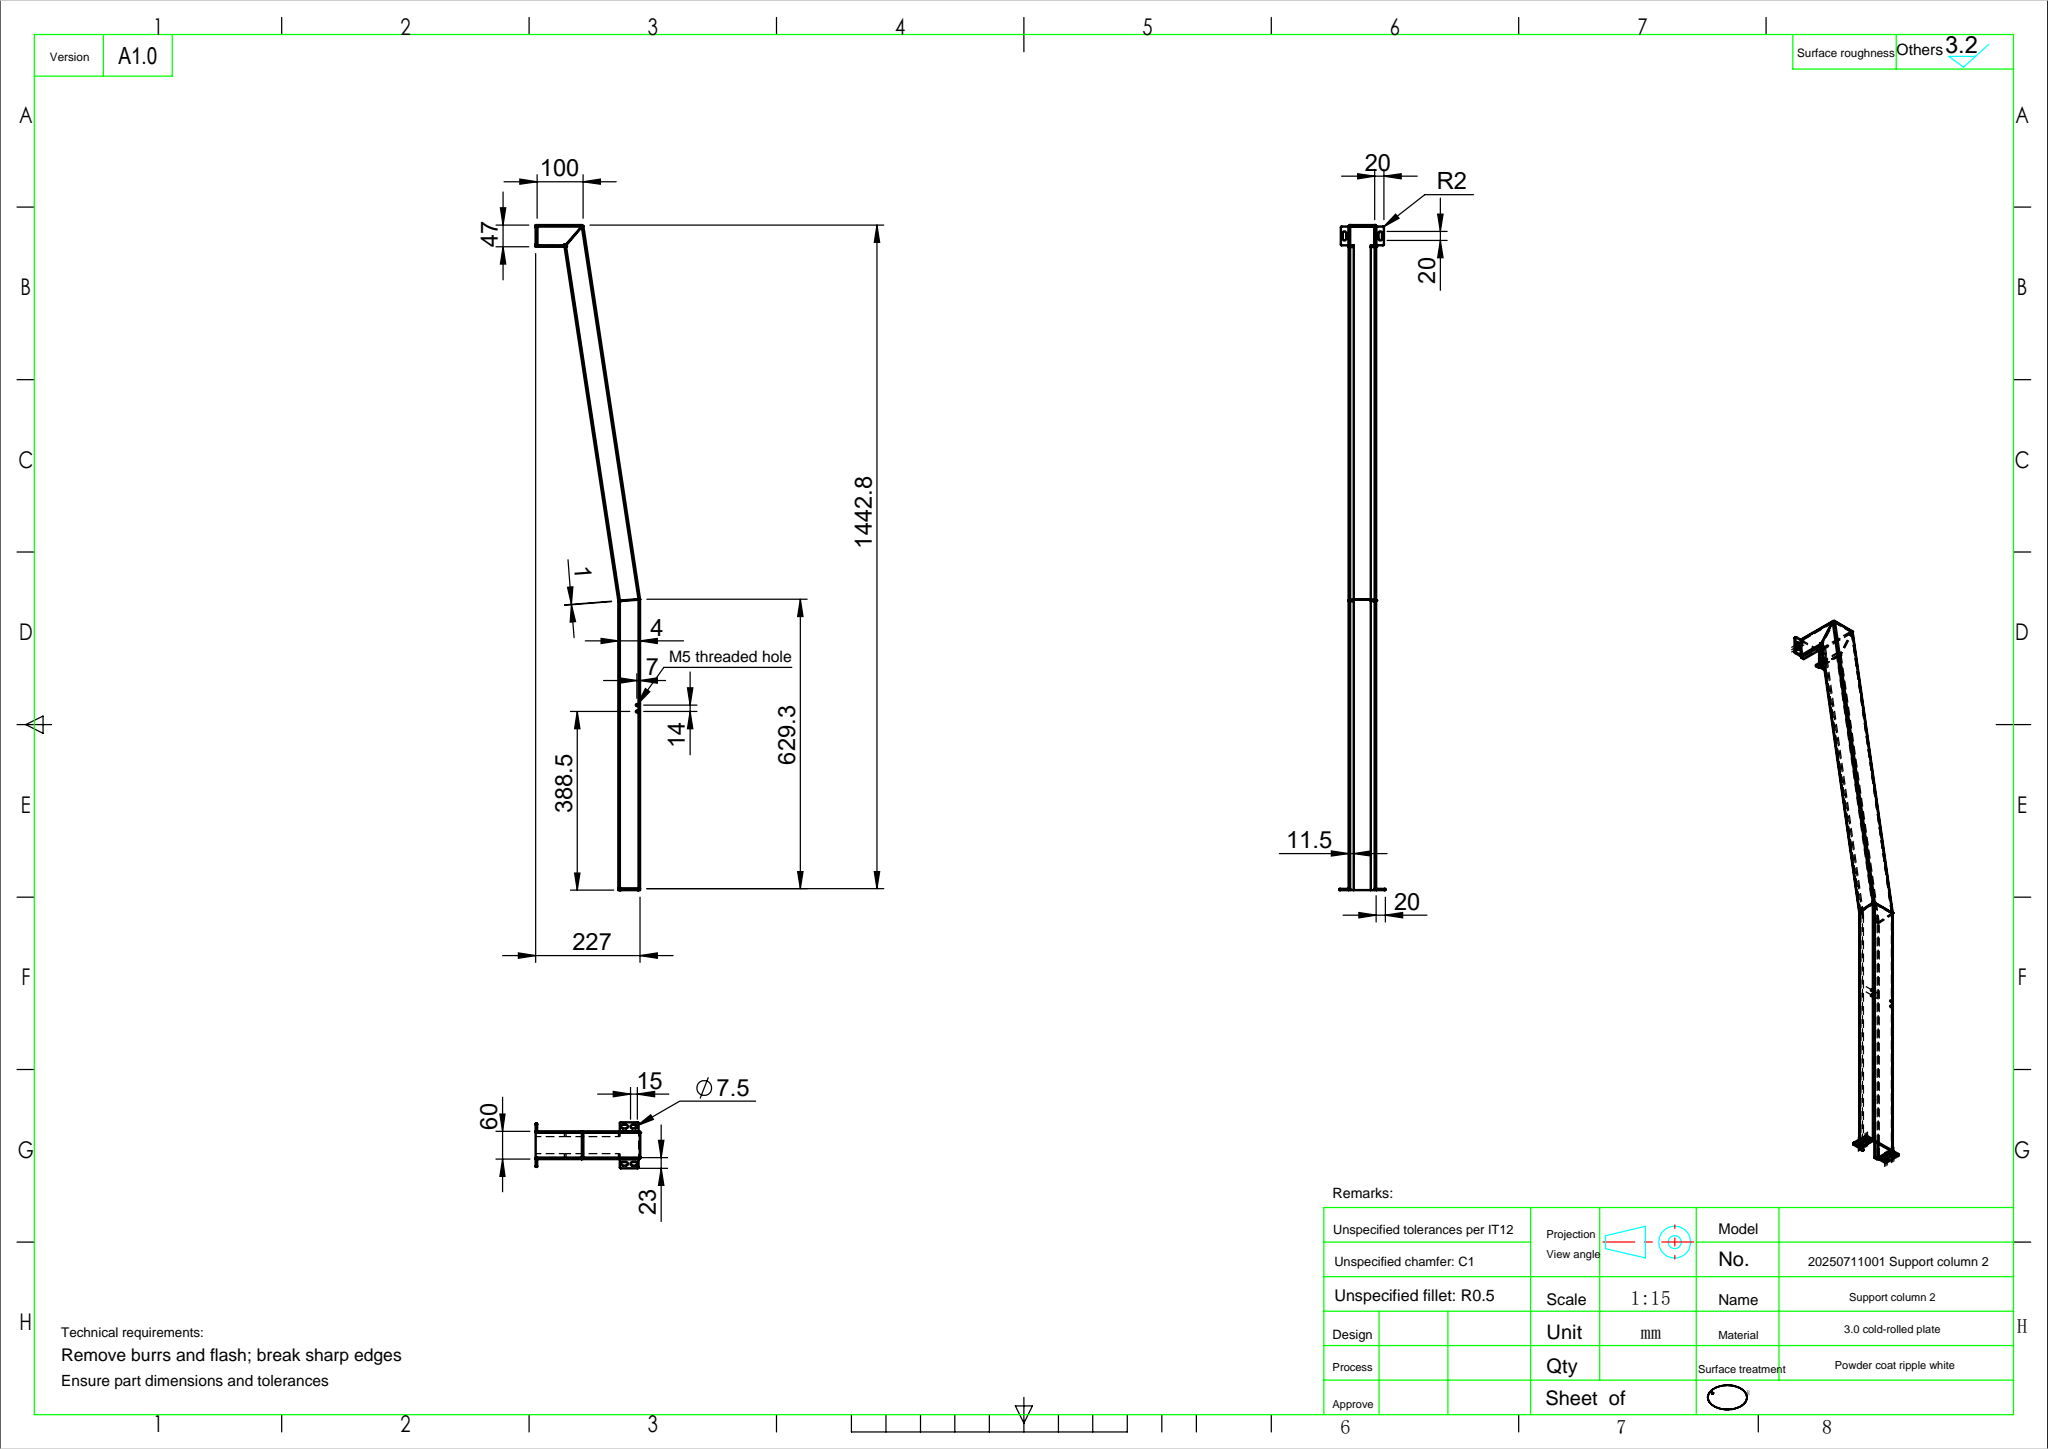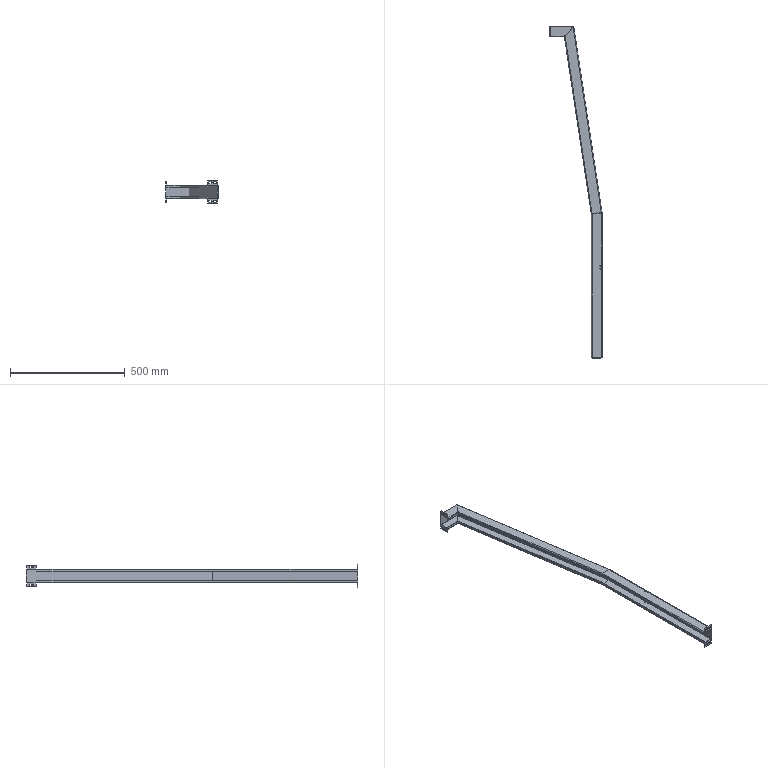Part | SolidWorks | features EdgeFlange 4, HoleWzd 3, CornerFeat 1, Fillet 1, FlatPattern 1, SMBaseFlange 1, SheetMetal 1 | 1 solid | 236 faces | box 227 x 1446 x 100 mm | volume 746223 mm3 | plane 150 | cylinder 76 | spline 10 | commonest cylinder face diameters 0.4 x18 6.4 x18 1.5 x12 7.5 x12 4 x8 4.2 x8